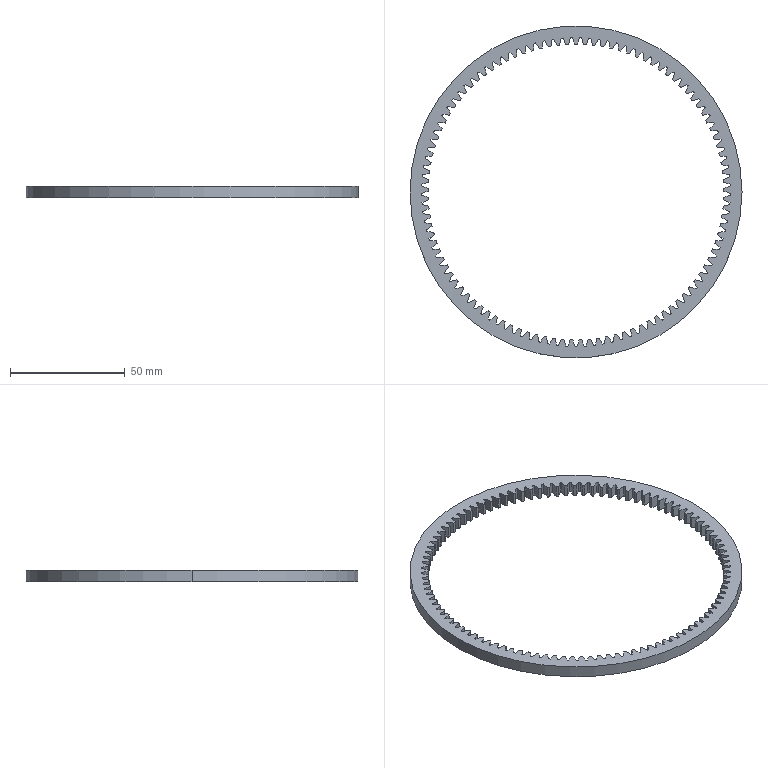Part | SolidWorks | features CirPattern 1, Extrusion 1, ICE 1, RefAxis 1 | 1 solid | 424 faces | box 144.5 x 144.5 x 5.2 mm | volume 14739 mm3 | cylinder 212 | spline 210 | plane 2 | commonest cylinder face diameters 128.755 x105 134.375 x105 144.5 x2